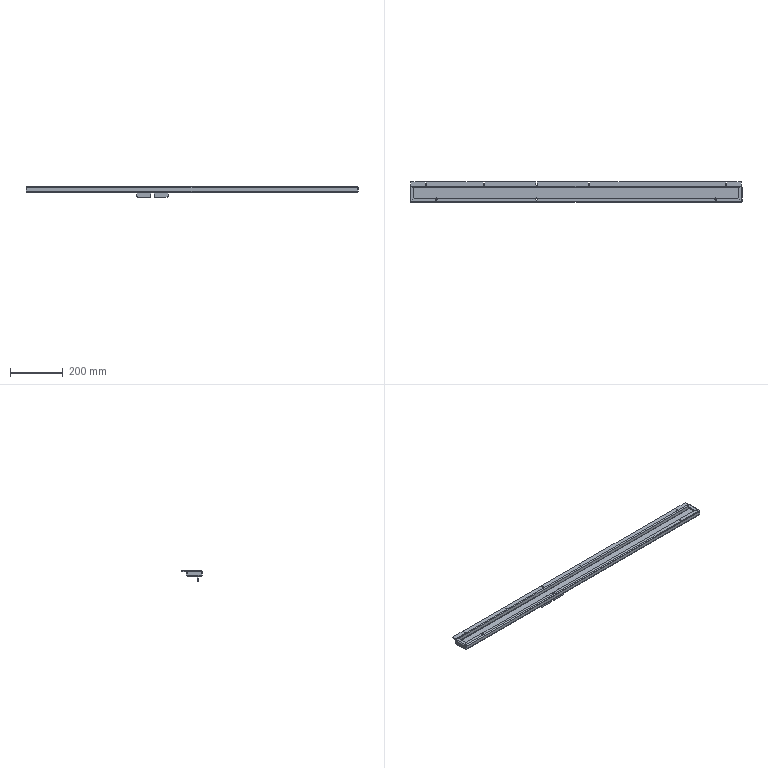Part | SolidWorks | features BaseBody 2 | 2 solids | 116 faces | box 1262 x 77 x 40 mm | volume 467224 mm3 | plane 63 | cylinder 41 | spline 12 | commonest cylinder face diameters 1.473 x10 7.473 x10 5.5 x6 12 x6 5.4 x4 10 x4